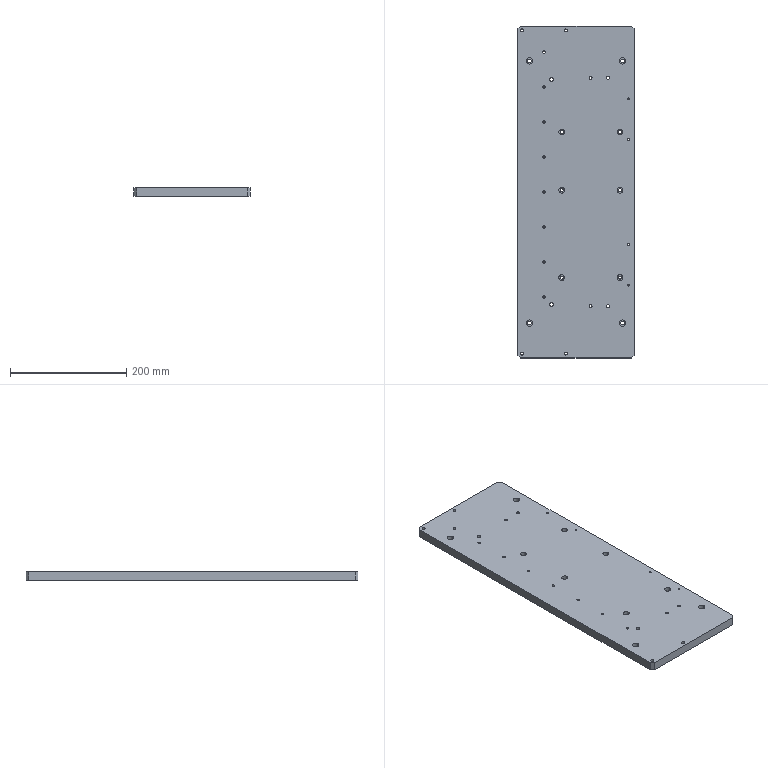Part | SolidWorks | features HoleWzd 8, Chamfer 1, Extrusion 1 | 1 solid | 104 faces | box 200 x 570 x 15 mm | volume 1695675 mm3 | cylinder 84 | plane 20 | commonest cylinder face diameters 4.2 x16 5 x16 5.5 x12 10 x12 3.3 x8 6.6 x8